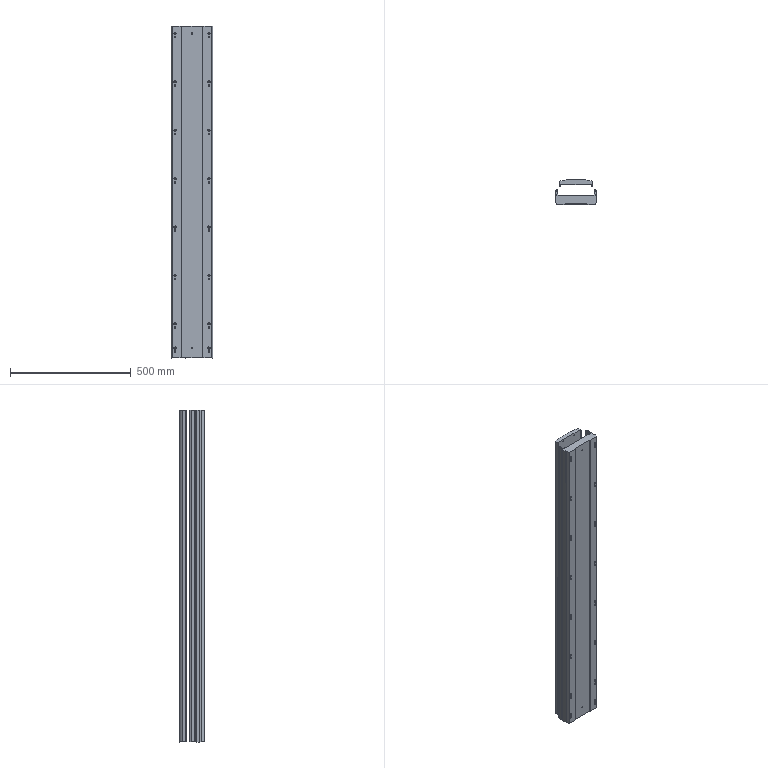Part | STEP file | 复件 FHB175-PRW-011^FHB175S-PRW-P40(马达RightUpper折-400W伺服电机) | 2 solids | 326 faces | box 170 x 103.1 x 1372 mm | volume 11406722 mm3 | cylinder 198 | plane 94 | cone 34 | commonest cylinder face diameters 0.6 x32 6.8 x32 9 x32 13.5 x32 10 x22 2 x15